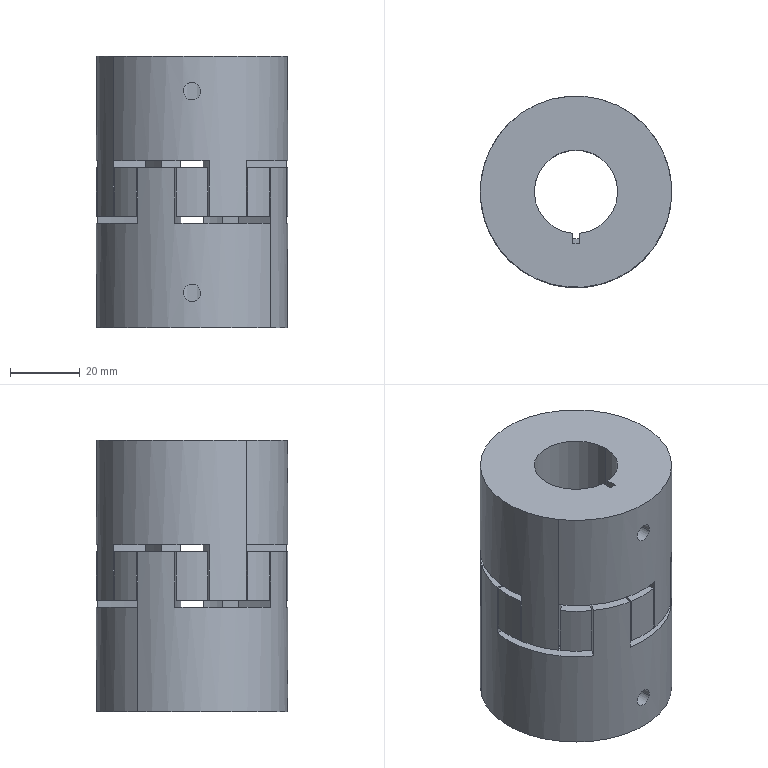Part | SolidWorks | features ICE 1, MBimport 1 | 3 solids | 100 faces | box 55 x 55 x 78 mm | volume 139645 mm3 | cylinder 74 | plane 26 | commonest cylinder face diameters 193.108 x16 194.108 x16 55 x12 31 x10 32 x8 24 x6